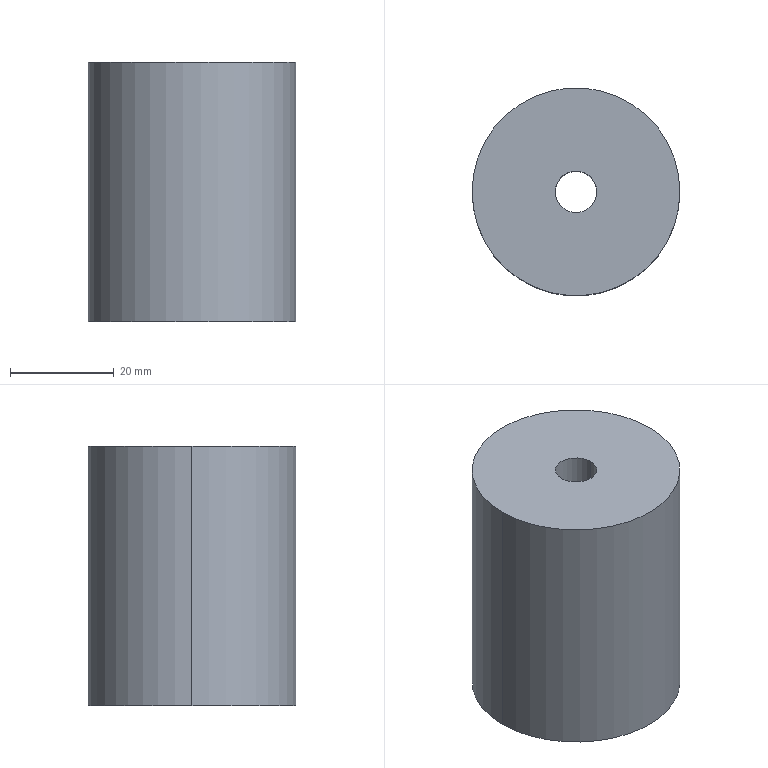Part | SolidWorks | features Extrusion 1 | 1 solid | 6 faces | box 40 x 40 x 50 mm | volume 60319 mm3 | cylinder 4 | plane 2 | commonest cylinder face diameters 8 x2 40 x2
STEP:
#1=CARTESIAN_POINT('',(-4.,0.,50.));
#2=VERTEX_POINT('',#1);
#3=CARTESIAN_POINT('',(4.,0.,50.));
#4=VERTEX_POINT('',#3);
#5=CARTESIAN_POINT('',(0.,0.,50.));
#6=DIRECTION('',(0.,0.,1.));
#7=DIRECTION('',(1.,0.,0.));
#8=AXIS2_PLACEMENT_3D('',#5,#6,#7);
#9=CIRCLE('',#8,4.);
#10=EDGE_CURVE('',#2,#4,#9,.T.);
#11=ORIENTED_EDGE('',*,*,#10,.T.);
#12=CARTESIAN_POINT('',(4.,0.,0.));
#13=VERTEX_POINT('',#12);
#14=CARTESIAN_POINT('',(4.,0.,50.));
#15=DIRECTION('',(0.,0.,-1.));
#16=VECTOR('',#15,1000.);
#17=LINE('',#14,#16);
#18=EDGE_CURVE('',#4,#13,#17,.T.);
#19=ORIENTED_EDGE('',*,*,#18,.T.);
#20=CARTESIAN_POINT('',(-4.,0.,0.));
#21=VERTEX_POINT('',#20);
#22=CARTESIAN_POINT('',(0.,0.,0.));
#23=DIRECTION('',(0.,0.,1.));
#24=DIRECTION('',(1.,0.,0.));
#25=AXIS2_PLACEMENT_3D('',#22,#23,#24);
#26=CIRCLE('',#25,4.);
#27=EDGE_CURVE('',#21,#13,#26,.T.);
#28=ORIENTED_EDGE('',*,*,#27,.F.);
#29=CARTESIAN_POINT('',(-4.,0.,50.));
#30=DIRECTION('',(0.,0.,-1.));
#31=VECTOR('',#30,1000.);
#32=LINE('',#29,#31);
#33=EDGE_CURVE('',#2,#21,#32,.T.);
#34=ORIENTED_EDGE('',*,*,#33,.F.);
#35=EDGE_LOOP('',(#11,#19,#28,#34));
#36=FACE_OUTER_BOUND('',#35,.T.);
#37=CARTESIAN_POINT('',(0.,0.,50.));
#38=DIRECTION('',(0.,0.,-1.));
#39=DIRECTION('',(-1.,0.,0.));
#40=AXIS2_PLACEMENT_3D('',#37,#38,#39);
#41=CYLINDRICAL_SURFACE('',#40,4.);
#42=ADVANCED_FACE('',(#36),#41,.F.);
#43=CARTESIAN_POINT('',(20.,0.,50.));
#44=VERTEX_POINT('',#43);
#45=CARTESIAN_POINT('',(-20.,0.,50.));
#46=VERTEX_POINT('',#45);
#47=CARTESIAN_POINT('',(0.,0.,50.));
#48=DIRECTION('',(0.,0.,1.));
#49=DIRECTION('',(1.,0.,0.));
#50=AXIS2_PLACEMENT_3D('',#47,#48,#49);
#51=CIRCLE('',#50,20.);
#52=EDGE_CURVE('',#44,#46,#51,.T.);
#53=ORIENTED_EDGE('',*,*,#52,.F.);
#54=CARTESIAN_POINT('',(20.,0.,0.));
#55=VERTEX_POINT('',#54);
#56=CARTESIAN_POINT('',(20.,0.,50.));
#57=DIRECTION('',(0.,0.,-1.));
#58=VECTOR('',#57,1000.);
#59=LINE('',#56,#58);
#60=EDGE_CURVE('',#44,#55,#59,.T.);
#61=ORIENTED_EDGE('',*,*,#60,.T.);
#62=CARTESIAN_POINT('',(-20.,0.,0.));
#63=VERTEX_POINT('',#62);
#64=CARTESIAN_POINT('',(0.,0.,0.));
#65=DIRECTION('',(0.,0.,1.));
#66=DIRECTION('',(1.,0.,0.));
#67=AXIS2_PLACEMENT_3D('',#64,#65,#66);
#68=CIRCLE('',#67,20.);
#69=EDGE_CURVE('',#55,#63,#68,.T.);
#70=ORIENTED_EDGE('',*,*,#69,.T.);
#71=CARTESIAN_POINT('',(-20.,0.,50.));
#72=DIRECTION('',(0.,0.,-1.));
#73=VECTOR('',#72,1000.);
#74=LINE('',#71,#73);
#75=EDGE_CURVE('',#46,#63,#74,.T.);
#76=ORIENTED_EDGE('',*,*,#75,.F.);
#77=EDGE_LOOP('',(#53,#61,#70,#76));
#78=FACE_OUTER_BOUND('',#77,.T.);
#79=CARTESIAN_POINT('',(0.,0.,50.));
#80=DIRECTION('',(0.,0.,-1.));
#81=DIRECTION('',(-1.,0.,0.));
#82=AXIS2_PLACEMENT_3D('',#79,#80,#81);
#83=CYLINDRICAL_SURFACE('',#82,20.);
#84=ADVANCED_FACE('',(#78),#83,.T.);
#85=CARTESIAN_POINT('',(0.,0.,50.));
#86=DIRECTION('',(0.,0.,1.));
#87=DIRECTION('',(1.,0.,0.));
#88=AXIS2_PLACEMENT_3D('',#85,#86,#87);
#89=CIRCLE('',#88,20.);
#90=EDGE_CURVE('',#46,#44,#89,.T.);
#91=ORIENTED_EDGE('',*,*,#90,.T.);
#92=ORIENTED_EDGE('',*,*,#52,.T.);
#93=EDGE_LOOP('',(#91,#92));
#94=FACE_OUTER_BOUND('',#93,.T.);
#95=ORIENTED_EDGE('',*,*,#10,.F.);
#96=CARTESIAN_POINT('',(0.,0.,50.));
#97=DIRECTION('',(0.,0.,1.));
#98=DIRECTION('',(1.,0.,0.));
#99=AXIS2_PLACEMENT_3D('',#96,#97,#98);
#100=CIRCLE('',#99,4.);
#101=EDGE_CURVE('',#4,#2,#100,.T.);
#102=ORIENTED_EDGE('',*,*,#101,.F.);
#103=EDGE_LOOP('',(#95,#102));
#104=FACE_BOUND('',#103,.T.);
#105=CARTESIAN_POINT('',(0.,0.,50.));
#106=DIRECTION('',(0.,0.,1.));
#107=DIRECTION('',(1.,0.,0.));
#108=AXIS2_PLACEMENT_3D('',#105,#106,#107);
#109=PLANE('',#108);
#110=ADVANCED_FACE('',(#94,#104),#109,.T.);
#111=CARTESIAN_POINT('',(0.,0.,0.));
#112=DIRECTION('',(0.,0.,1.));
#113=DIRECTION('',(1.,0.,0.));
#114=AXIS2_PLACEMENT_3D('',#111,#112,#113);
#115=CIRCLE('',#114,20.);
#116=EDGE_CURVE('',#63,#55,#115,.T.);
#117=ORIENTED_EDGE('',*,*,#116,.F.);
#118=ORIENTED_EDGE('',*,*,#69,.F.);
#119=EDGE_LOOP('',(#117,#118));
#120=FACE_OUTER_BOUND('',#119,.T.);
#121=ORIENTED_EDGE('',*,*,#27,.T.);
#122=CARTESIAN_POINT('',(0.,0.,0.));
#123=DIRECTION('',(0.,0.,1.));
#124=DIRECTION('',(1.,0.,0.));
#125=AXIS2_PLACEMENT_3D('',#122,#123,#124);
#126=CIRCLE('',#125,4.);
#127=EDGE_CURVE('',#13,#21,#126,.T.);
#128=ORIENTED_EDGE('',*,*,#127,.T.);
#129=EDGE_LOOP('',(#121,#128));
#130=FACE_BOUND('',#129,.T.);
#131=CARTESIAN_POINT('',(0.,0.,0.));
#132=DIRECTION('',(0.,0.,1.));
#133=DIRECTION('',(1.,0.,0.));
#134=AXIS2_PLACEMENT_3D('',#131,#132,#133);
#135=PLANE('',#134);
#136=ADVANCED_FACE('',(#120,#130),#135,.F.);
#137=ORIENTED_EDGE('',*,*,#60,.F.);
#138=ORIENTED_EDGE('',*,*,#90,.F.);
#139=ORIENTED_EDGE('',*,*,#75,.T.);
#140=ORIENTED_EDGE('',*,*,#116,.T.);
#141=EDGE_LOOP('',(#137,#138,#139,#140));
#142=FACE_OUTER_BOUND('',#141,.T.);
#143=CARTESIAN_POINT('',(0.,0.,50.));
#144=DIRECTION('',(0.,0.,-1.));
#145=DIRECTION('',(-1.,0.,0.));
#146=AXIS2_PLACEMENT_3D('',#143,#144,#145);
#147=CYLINDRICAL_SURFACE('',#146,20.);
#148=ADVANCED_FACE('',(#142),#147,.T.);
#149=ORIENTED_EDGE('',*,*,#18,.F.);
#150=ORIENTED_EDGE('',*,*,#101,.T.);
#151=ORIENTED_EDGE('',*,*,#33,.T.);
#152=ORIENTED_EDGE('',*,*,#127,.F.);
#153=EDGE_LOOP('',(#149,#150,#151,#152));
#154=FACE_OUTER_BOUND('',#153,.T.);
#155=CARTESIAN_POINT('',(0.,0.,50.));
#156=DIRECTION('',(0.,0.,-1.));
#157=DIRECTION('',(-1.,0.,0.));
#158=AXIS2_PLACEMENT_3D('',#155,#156,#157);
#159=CYLINDRICAL_SURFACE('',#158,4.);
#160=ADVANCED_FACE('',(#154),#159,.F.);
#161=CLOSED_SHELL('',(#42,#84,#110,#136,#148,#160));
#162=MANIFOLD_SOLID_BREP('',#161);
#163=CARTESIAN_POINT('',(0.,0.,0.));
#164=DIRECTION('',(0.,0.,1.));
#165=DIRECTION('',(1.,0.,0.));
#166=AXIS2_PLACEMENT_3D('',#163,#164,#165);
#167=(LENGTH_UNIT()NAMED_UNIT(*)SI_UNIT(.MILLI.,.METRE.));
#168=UNCERTAINTY_MEASURE_WITH_UNIT(LENGTH_MEASURE(0.00001),#167,'','');
#169=(NAMED_UNIT(*)PLANE_ANGLE_UNIT()SI_UNIT($,.RADIAN.));
#170=(NAMED_UNIT(*)SI_UNIT($,.STERADIAN.)SOLID_ANGLE_UNIT());
#171=(GEOMETRIC_REPRESENTATION_CONTEXT(3)GLOBAL_UNCERTAINTY_ASSIGNED_CONTEXT((#168))GLOBAL_UNIT_ASSIGNED_CONTEXT((#167,#169,#170))REPRESENTATION_CONTEXT('',''));
#172=ADVANCED_BREP_SHAPE_REPRESENTATION('',(#162,#166),#171);